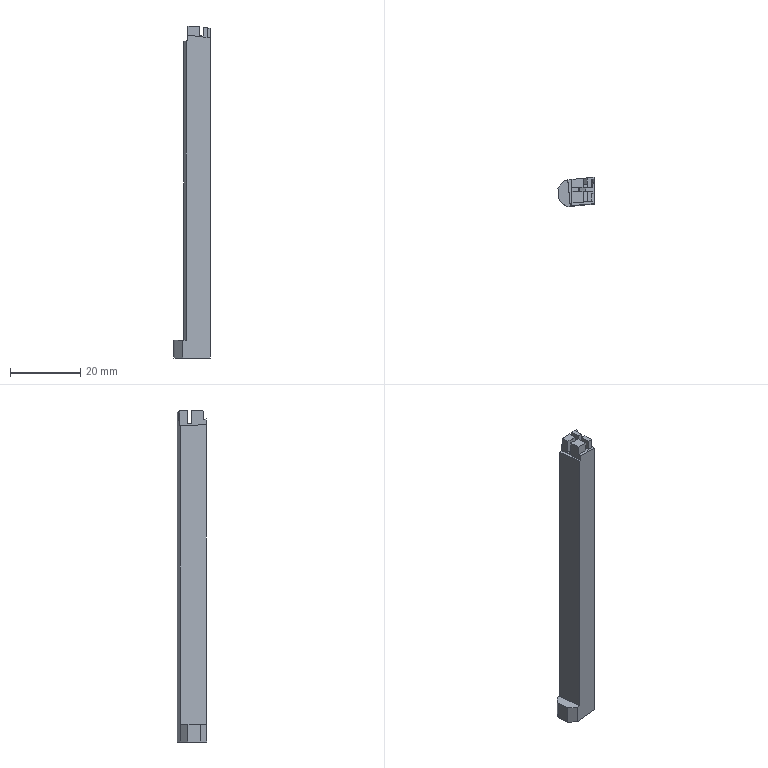Part | STEP file | P011002M011-000 | 1 solid | 43 faces | box 10.289 x 8.281 x 94.692 mm | volume 4991 mm3 | spline 35 | plane 8